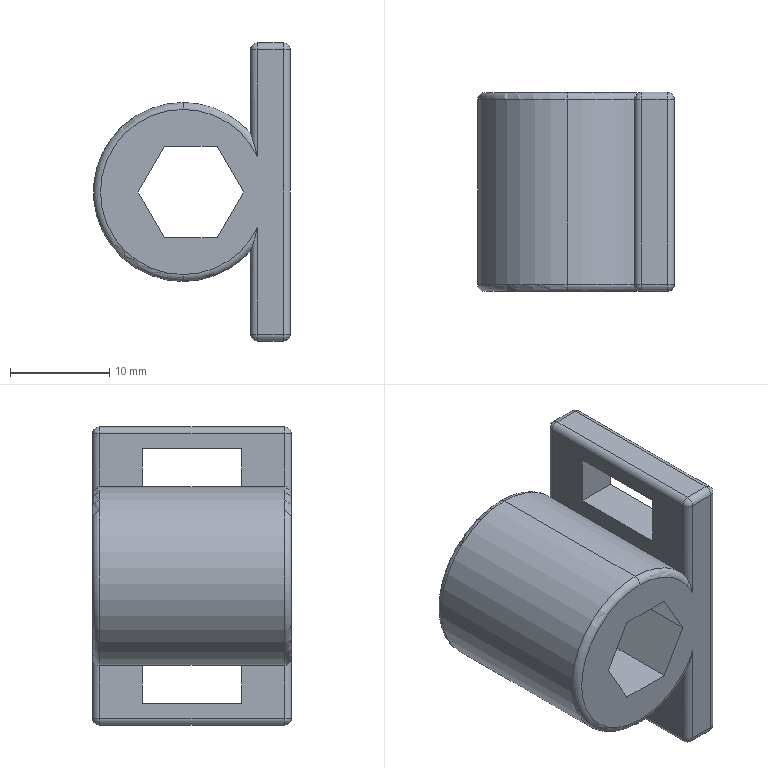Part | SolidWorks | features ICE 3, Fillet 2, Extrusion 1, MirrorPattern 1 | 1 solid | 52 faces | box 19.787 x 20 x 30 mm | volume 5242 mm3 | plane 21 | cylinder 17 | sphere 8 | torus 6 | commonest cylinder face diameters 1.4 x14 18 x3
STEP:
#1=CARTESIAN_POINT('',(-0.787,9.3,-9.));
#2=VERTEX_POINT('',#1);
#3=CARTESIAN_POINT('',(6.,9.3,-5.911));
#4=VERTEX_POINT('',#3);
#5=CARTESIAN_POINT('',(-0.787,9.3,0.));
#6=DIRECTION('',(0.,-1.,0.));
#7=DIRECTION('',(0.,0.,1.));
#8=AXIS2_PLACEMENT_3D('',#5,#6,#7);
#9=CIRCLE('',#8,9.);
#10=EDGE_CURVE('',#2,#4,#9,.T.);
#11=ORIENTED_EDGE('',*,*,#10,.F.);
#12=CARTESIAN_POINT('',(-0.787,10.,-8.3));
#13=VERTEX_POINT('',#12);
#14=CARTESIAN_POINT('',(-0.787,9.3,-8.3));
#15=DIRECTION('',(1.,0.,0.));
#16=DIRECTION('',(0.,0.,-1.));
#17=AXIS2_PLACEMENT_3D('',#14,#15,#16);
#18=CIRCLE('',#17,0.7);
#19=EDGE_CURVE('',#2,#13,#18,.T.);
#20=ORIENTED_EDGE('',*,*,#19,.T.);
#21=CARTESIAN_POINT('',(6.7,10.,-3.583));
#22=VERTEX_POINT('',#21);
#23=CARTESIAN_POINT('',(-0.787,10.,0.));
#24=DIRECTION('',(0.,1.,0.));
#25=DIRECTION('',(0.,0.,1.));
#26=AXIS2_PLACEMENT_3D('',#23,#24,#25);
#27=CIRCLE('',#26,8.3);
#28=EDGE_CURVE('',#22,#13,#27,.T.);
#29=ORIENTED_EDGE('',*,*,#28,.F.);
#30=CARTESIAN_POINT('',(6.,9.3,-5.911));
#31=CARTESIAN_POINT('',(6.,9.357,-5.911));
#32=CARTESIAN_POINT('',(6.007,9.412,-5.891));
#33=CARTESIAN_POINT('',(6.029,9.505,-5.833));
#34=CARTESIAN_POINT('',(6.043,9.545,-5.794));
#35=CARTESIAN_POINT('',(6.089,9.649,-5.67));
#36=CARTESIAN_POINT('',(6.123,9.699,-5.575));
#37=CARTESIAN_POINT('',(6.224,9.824,-5.283));
#38=CARTESIAN_POINT('',(6.293,9.874,-5.074));
#39=CARTESIAN_POINT('',(6.421,9.946,-4.656));
#40=CARTESIAN_POINT('',(6.482,9.968,-4.444));
#41=CARTESIAN_POINT('',(6.597,9.995,-4.016));
#42=CARTESIAN_POINT('',(6.65,10.,-3.802));
#43=CARTESIAN_POINT('',(6.7,10.,-3.583));
#44=B_SPLINE_CURVE_WITH_KNOTS('',3,(#30,#31,#32,#33,#34,#35,#36,#37,#38,#39,#40,#41,#42,#43),.UNSPECIFIED.,.F.,.F.,(4,2,2,2,2,2,4),(0.,0.0001684,0.0003368,0.0006737,0.001347,0.002021,0.002695),.UNSPECIFIED.);
#45=EDGE_CURVE('',#4,#22,#44,.T.);
#46=ORIENTED_EDGE('',*,*,#45,.F.);
#47=EDGE_LOOP('',(#11,#20,#29,#46));
#48=FACE_OUTER_BOUND('',#47,.T.);
#49=CARTESIAN_POINT('',(-0.787,9.3,0.));
#50=DIRECTION('',(0.,1.,0.));
#51=DIRECTION('',(0.,0.,1.));
#52=AXIS2_PLACEMENT_3D('',#49,#50,#51);
#53=TOROIDAL_SURFACE('',#52,8.3,0.7);
#54=ADVANCED_FACE('',(#48),#53,.T.);
#55=ORIENTED_EDGE('',*,*,#19,.F.);
#56=CARTESIAN_POINT('',(-0.787,9.3,9.));
#57=VERTEX_POINT('',#56);
#58=CARTESIAN_POINT('',(-0.787,9.3,0.));
#59=DIRECTION('',(0.,-1.,0.));
#60=DIRECTION('',(0.,0.,1.));
#61=AXIS2_PLACEMENT_3D('',#58,#59,#60);
#62=CIRCLE('',#61,9.);
#63=EDGE_CURVE('',#57,#2,#62,.T.);
#64=ORIENTED_EDGE('',*,*,#63,.F.);
#65=CARTESIAN_POINT('',(-0.787,10.,8.3));
#66=VERTEX_POINT('',#65);
#67=CARTESIAN_POINT('',(-0.787,9.3,8.3));
#68=DIRECTION('',(-1.,0.,0.));
#69=DIRECTION('',(0.,0.,1.));
#70=AXIS2_PLACEMENT_3D('',#67,#68,#69);
#71=CIRCLE('',#70,0.7);
#72=EDGE_CURVE('',#57,#66,#71,.T.);
#73=ORIENTED_EDGE('',*,*,#72,.T.);
#74=CARTESIAN_POINT('',(-0.787,10.,0.));
#75=DIRECTION('',(0.,1.,0.));
#76=DIRECTION('',(0.,0.,1.));
#77=AXIS2_PLACEMENT_3D('',#74,#75,#76);
#78=CIRCLE('',#77,8.3);
#79=EDGE_CURVE('',#13,#66,#78,.T.);
#80=ORIENTED_EDGE('',*,*,#79,.F.);
#81=EDGE_LOOP('',(#55,#64,#73,#80));
#82=FACE_OUTER_BOUND('',#81,.T.);
#83=CARTESIAN_POINT('',(-0.787,9.3,0.));
#84=DIRECTION('',(0.,1.,0.));
#85=DIRECTION('',(0.,0.,1.));
#86=AXIS2_PLACEMENT_3D('',#83,#84,#85);
#87=TOROIDAL_SURFACE('',#86,8.3,0.7);
#88=ADVANCED_FACE('',(#82),#87,.T.);
#89=CARTESIAN_POINT('',(-0.787,-10.,-8.3));
#90=VERTEX_POINT('',#89);
#91=CARTESIAN_POINT('',(6.7,-10.,-3.583));
#92=VERTEX_POINT('',#91);
#93=CARTESIAN_POINT('',(-0.787,-10.,0.));
#94=DIRECTION('',(0.,-1.,0.));
#95=DIRECTION('',(0.,0.,1.));
#96=AXIS2_PLACEMENT_3D('',#93,#94,#95);
#97=CIRCLE('',#96,8.3);
#98=EDGE_CURVE('',#90,#92,#97,.T.);
#99=ORIENTED_EDGE('',*,*,#98,.F.);
#100=CARTESIAN_POINT('',(-0.787,-9.3,-9.));
#101=VERTEX_POINT('',#100);
#102=CARTESIAN_POINT('',(-0.787,-9.3,-8.3));
#103=DIRECTION('',(1.,0.,0.));
#104=DIRECTION('',(0.,0.,-1.));
#105=AXIS2_PLACEMENT_3D('',#102,#103,#104);
#106=CIRCLE('',#105,0.7);
#107=EDGE_CURVE('',#90,#101,#106,.T.);
#108=ORIENTED_EDGE('',*,*,#107,.T.);
#109=CARTESIAN_POINT('',(6.,-9.3,-5.911));
#110=VERTEX_POINT('',#109);
#111=CARTESIAN_POINT('',(-0.787,-9.3,0.));
#112=DIRECTION('',(0.,1.,0.));
#113=DIRECTION('',(0.,0.,1.));
#114=AXIS2_PLACEMENT_3D('',#111,#112,#113);
#115=CIRCLE('',#114,9.);
#116=EDGE_CURVE('',#110,#101,#115,.T.);
#117=ORIENTED_EDGE('',*,*,#116,.F.);
#118=CARTESIAN_POINT('',(6.7,-10.,-3.583));
#119=CARTESIAN_POINT('',(6.601,-10.,-4.017));
#120=CARTESIAN_POINT('',(6.486,-9.983,-4.447));
#121=CARTESIAN_POINT('',(6.293,-9.874,-5.074));
#122=CARTESIAN_POINT('',(6.224,-9.824,-5.283));
#123=CARTESIAN_POINT('',(6.123,-9.699,-5.575));
#124=CARTESIAN_POINT('',(6.089,-9.649,-5.67));
#125=CARTESIAN_POINT('',(6.043,-9.545,-5.794));
#126=CARTESIAN_POINT('',(6.029,-9.505,-5.833));
#127=CARTESIAN_POINT('',(6.007,-9.412,-5.891));
#128=CARTESIAN_POINT('',(6.,-9.357,-5.911));
#129=CARTESIAN_POINT('',(6.,-9.3,-5.911));
#130=B_SPLINE_CURVE_WITH_KNOTS('',3,(#118,#119,#120,#121,#122,#123,#124,#125,#126,#127,#128,#129),.UNSPECIFIED.,.F.,.F.,(4,2,2,2,2,4),(-0.000008054,0.001327,0.001995,0.002329,0.002496,0.002663),.UNSPECIFIED.);
#131=EDGE_CURVE('',#92,#110,#130,.T.);
#132=ORIENTED_EDGE('',*,*,#131,.F.);
#133=EDGE_LOOP('',(#99,#108,#117,#132));
#134=FACE_OUTER_BOUND('',#133,.T.);
#135=CARTESIAN_POINT('',(-0.787,-9.3,0.));
#136=DIRECTION('',(0.,1.,0.));
#137=DIRECTION('',(0.,0.,1.));
#138=AXIS2_PLACEMENT_3D('',#135,#136,#137);
#139=TOROIDAL_SURFACE('',#138,8.3,0.7);
#140=ADVANCED_FACE('',(#134),#139,.T.);
#141=ORIENTED_EDGE('',*,*,#107,.F.);
#142=CARTESIAN_POINT('',(-0.787,-10.,8.3));
#143=VERTEX_POINT('',#142);
#144=CARTESIAN_POINT('',(-0.787,-10.,0.));
#145=DIRECTION('',(0.,-1.,0.));
#146=DIRECTION('',(0.,0.,1.));
#147=AXIS2_PLACEMENT_3D('',#144,#145,#146);
#148=CIRCLE('',#147,8.3);
#149=EDGE_CURVE('',#143,#90,#148,.T.);
#150=ORIENTED_EDGE('',*,*,#149,.F.);
#151=CARTESIAN_POINT('',(-0.787,-9.3,9.));
#152=VERTEX_POINT('',#151);
#153=CARTESIAN_POINT('',(-0.787,-9.3,8.3));
#154=DIRECTION('',(-1.,0.,0.));
#155=DIRECTION('',(0.,0.,1.));
#156=AXIS2_PLACEMENT_3D('',#153,#154,#155);
#157=CIRCLE('',#156,0.7);
#158=EDGE_CURVE('',#143,#152,#157,.T.);
#159=ORIENTED_EDGE('',*,*,#158,.T.);
#160=CARTESIAN_POINT('',(-0.787,-9.3,0.));
#161=DIRECTION('',(0.,1.,0.));
#162=DIRECTION('',(0.,0.,1.));
#163=AXIS2_PLACEMENT_3D('',#160,#161,#162);
#164=CIRCLE('',#163,9.);
#165=EDGE_CURVE('',#101,#152,#164,.T.);
#166=ORIENTED_EDGE('',*,*,#165,.F.);
#167=EDGE_LOOP('',(#141,#150,#159,#166));
#168=FACE_OUTER_BOUND('',#167,.T.);
#169=CARTESIAN_POINT('',(-0.787,-9.3,0.));
#170=DIRECTION('',(0.,1.,0.));
#171=DIRECTION('',(0.,0.,1.));
#172=AXIS2_PLACEMENT_3D('',#169,#170,#171);
#173=TOROIDAL_SURFACE('',#172,8.3,0.7);
#174=ADVANCED_FACE('',(#168),#173,.T.);
#175=ORIENTED_EDGE('',*,*,#116,.T.);
#176=CARTESIAN_POINT('',(-0.787,-10.,-9.));
#177=DIRECTION('',(0.,1.,0.));
#178=VECTOR('',#177,1000.);
#179=LINE('',#176,#178);
#180=EDGE_CURVE('',#101,#2,#179,.T.);
#181=ORIENTED_EDGE('',*,*,#180,.T.);
#182=ORIENTED_EDGE('',*,*,#10,.T.);
#183=CARTESIAN_POINT('',(6.,-10.,-5.911));
#184=DIRECTION('',(0.,1.,0.));
#185=VECTOR('',#184,1000.);
#186=LINE('',#183,#185);
#187=EDGE_CURVE('',#110,#4,#186,.T.);
#188=ORIENTED_EDGE('',*,*,#187,.F.);
#189=EDGE_LOOP('',(#175,#181,#182,#188));
#190=FACE_OUTER_BOUND('',#189,.T.);
#191=CARTESIAN_POINT('',(-0.787,-10.,0.));
#192=DIRECTION('',(0.,1.,0.));
#193=DIRECTION('',(0.,0.,1.));
#194=AXIS2_PLACEMENT_3D('',#191,#192,#193);
#195=CYLINDRICAL_SURFACE('',#194,9.);
#196=ADVANCED_FACE('',(#190),#195,.T.);
#197=ORIENTED_EDGE('',*,*,#180,.F.);
#198=ORIENTED_EDGE('',*,*,#165,.T.);
#199=CARTESIAN_POINT('',(-0.787,-10.,9.));
#200=DIRECTION('',(0.,1.,0.));
#201=VECTOR('',#200,1000.);
#202=LINE('',#199,#201);
#203=EDGE_CURVE('',#152,#57,#202,.T.);
#204=ORIENTED_EDGE('',*,*,#203,.T.);
#205=ORIENTED_EDGE('',*,*,#63,.T.);
#206=EDGE_LOOP('',(#197,#198,#204,#205));
#207=FACE_OUTER_BOUND('',#206,.T.);
#208=CARTESIAN_POINT('',(-0.787,-10.,0.));
#209=DIRECTION('',(0.,1.,0.));
#210=DIRECTION('',(0.,0.,1.));
#211=AXIS2_PLACEMENT_3D('',#208,#209,#210);
#212=CYLINDRICAL_SURFACE('',#211,9.);
#213=ADVANCED_FACE('',(#207),#212,.T.);
#214=CARTESIAN_POINT('',(10.,-9.3,-14.3));
#215=VERTEX_POINT('',#214);
#216=CARTESIAN_POINT('',(10.,9.3,-14.3));
#217=VERTEX_POINT('',#216);
#218=CARTESIAN_POINT('',(10.,10.,-14.3));
#219=DIRECTION('',(0.,1.,0.));
#220=VECTOR('',#219,1000.);
#221=LINE('',#218,#220);
#222=EDGE_CURVE('',#215,#217,#221,.T.);
#223=ORIENTED_EDGE('',*,*,#222,.T.);
#224=CARTESIAN_POINT('',(10.,9.3,14.3));
#225=VERTEX_POINT('',#224);
#226=CARTESIAN_POINT('',(10.,9.3,15.));
#227=DIRECTION('',(0.,0.,1.));
#228=VECTOR('',#227,1000.);
#229=LINE('',#226,#228);
#230=EDGE_CURVE('',#217,#225,#229,.T.);
#231=ORIENTED_EDGE('',*,*,#230,.T.);
#232=CARTESIAN_POINT('',(10.,-9.3,14.3));
#233=VERTEX_POINT('',#232);
#234=CARTESIAN_POINT('',(10.,10.,14.3));
#235=DIRECTION('',(0.,-1.,0.));
#236=VECTOR('',#235,1000.);
#237=LINE('',#234,#236);
#238=EDGE_CURVE('',#225,#233,#237,.T.);
#239=ORIENTED_EDGE('',*,*,#238,.T.);
#240=CARTESIAN_POINT('',(10.,-9.3,-15.));
#241=DIRECTION('',(0.,0.,-1.));
#242=VECTOR('',#241,1000.);
#243=LINE('',#240,#242);
#244=EDGE_CURVE('',#233,#215,#243,.T.);
#245=ORIENTED_EDGE('',*,*,#244,.T.);
#246=EDGE_LOOP('',(#223,#231,#239,#245));
#247=FACE_OUTER_BOUND('',#246,.T.);
#248=CARTESIAN_POINT('',(10.,5.,12.8));
#249=VERTEX_POINT('',#248);
#250=CARTESIAN_POINT('',(10.,5.,7.8));
#251=VERTEX_POINT('',#250);
#252=CARTESIAN_POINT('',(10.,5.,-15.));
#253=DIRECTION('',(0.,0.,-1.));
#254=VECTOR('',#253,1000.);
#255=LINE('',#252,#254);
#256=EDGE_CURVE('',#249,#251,#255,.T.);
#257=ORIENTED_EDGE('',*,*,#256,.T.);
#258=CARTESIAN_POINT('',(10.,-5.,7.8));
#259=VERTEX_POINT('',#258);
#260=CARTESIAN_POINT('',(10.,10.,7.8));
#261=DIRECTION('',(0.,-1.,0.));
#262=VECTOR('',#261,1000.);
#263=LINE('',#260,#262);
#264=EDGE_CURVE('',#251,#259,#263,.T.);
#265=ORIENTED_EDGE('',*,*,#264,.T.);
#266=CARTESIAN_POINT('',(10.,-5.,12.8));
#267=VERTEX_POINT('',#266);
#268=CARTESIAN_POINT('',(10.,-5.,-15.));
#269=DIRECTION('',(0.,0.,1.));
#270=VECTOR('',#269,1000.);
#271=LINE('',#268,#270);
#272=EDGE_CURVE('',#259,#267,#271,.T.);
#273=ORIENTED_EDGE('',*,*,#272,.T.);
#274=CARTESIAN_POINT('',(10.,10.,12.8));
#275=DIRECTION('',(0.,1.,0.));
#276=VECTOR('',#275,1000.);
#277=LINE('',#274,#276);
#278=EDGE_CURVE('',#267,#249,#277,.T.);
#279=ORIENTED_EDGE('',*,*,#278,.T.);
#280=EDGE_LOOP('',(#257,#265,#273,#279));
#281=FACE_BOUND('',#280,.T.);
#282=CARTESIAN_POINT('',(10.,5.,-7.8));
#283=VERTEX_POINT('',#282);
#284=CARTESIAN_POINT('',(10.,-5.,-7.8));
#285=VERTEX_POINT('',#284);
#286=CARTESIAN_POINT('',(10.,10.,-7.8));
#287=DIRECTION('',(0.,-1.,0.));
#288=VECTOR('',#287,1000.);
#289=LINE('',#286,#288);
#290=EDGE_CURVE('',#283,#285,#289,.T.);
#291=ORIENTED_EDGE('',*,*,#290,.F.);
#292=CARTESIAN_POINT('',(10.,5.,-12.8));
#293=VERTEX_POINT('',#292);
#294=CARTESIAN_POINT('',(10.,5.,-15.));
#295=DIRECTION('',(0.,0.,1.));
#296=VECTOR('',#295,1000.);
#297=LINE('',#294,#296);
#298=EDGE_CURVE('',#293,#283,#297,.T.);
#299=ORIENTED_EDGE('',*,*,#298,.F.);
#300=CARTESIAN_POINT('',(10.,-5.,-12.8));
#301=VERTEX_POINT('',#300);
#302=CARTESIAN_POINT('',(10.,10.,-12.8));
#303=DIRECTION('',(0.,1.,0.));
#304=VECTOR('',#303,1000.);
#305=LINE('',#302,#304);
#306=EDGE_CURVE('',#301,#293,#305,.T.);
#307=ORIENTED_EDGE('',*,*,#306,.F.);
#308=CARTESIAN_POINT('',(10.,-5.,-15.));
#309=DIRECTION('',(0.,0.,-1.));
#310=VECTOR('',#309,1000.);
#311=LINE('',#308,#310);
#312=EDGE_CURVE('',#285,#301,#311,.T.);
#313=ORIENTED_EDGE('',*,*,#312,.F.);
#314=EDGE_LOOP('',(#291,#299,#307,#313));
#315=FACE_BOUND('',#314,.T.);
#316=CARTESIAN_POINT('',(10.,10.,-15.));
#317=DIRECTION('',(-1.,0.,0.));
#318=DIRECTION('',(0.,0.,1.));
#319=AXIS2_PLACEMENT_3D('',#316,#317,#318);
#320=PLANE('',#319);
#321=ADVANCED_FACE('',(#247,#281,#315),#320,.F.);
#322=CARTESIAN_POINT('',(6.,9.3,-14.3));
#323=VERTEX_POINT('',#322);
#324=CARTESIAN_POINT('',(6.,-9.3,-14.3));
#325=VERTEX_POINT('',#324);
#326=CARTESIAN_POINT('',(6.,-10.,-14.3));
#327=DIRECTION('',(0.,-1.,0.));
#328=VECTOR('',#327,1000.);
#329=LINE('',#326,#328);
#330=EDGE_CURVE('',#323,#325,#329,.T.);
#331=ORIENTED_EDGE('',*,*,#330,.T.);
#332=CARTESIAN_POINT('',(6.,-9.3,-5.911));
#333=DIRECTION('',(0.,0.,1.));
#334=VECTOR('',#333,1000.);
#335=LINE('',#332,#334);
#336=EDGE_CURVE('',#325,#110,#335,.T.);
#337=ORIENTED_EDGE('',*,*,#336,.T.);
#338=ORIENTED_EDGE('',*,*,#187,.T.);
#339=CARTESIAN_POINT('',(6.,9.3,-5.911));
#340=DIRECTION('',(0.,0.,-1.));
#341=VECTOR('',#340,1000.);
#342=LINE('',#339,#341);
#343=EDGE_CURVE('',#4,#323,#342,.T.);
#344=ORIENTED_EDGE('',*,*,#343,.T.);
#345=EDGE_LOOP('',(#331,#337,#338,#344));
#346=FACE_OUTER_BOUND('',#345,.T.);
#347=CARTESIAN_POINT('',(6.,5.,-12.8));
#348=VERTEX_POINT('',#347);
#349=CARTESIAN_POINT('',(6.,5.,-7.8));
#350=VERTEX_POINT('',#349);
#351=CARTESIAN_POINT('',(6.,5.,-7.8));
#352=DIRECTION('',(0.,0.,1.));
#353=VECTOR('',#352,1000.);
#354=LINE('',#351,#353);
#355=EDGE_CURVE('',#348,#350,#354,.T.);
#356=ORIENTED_EDGE('',*,*,#355,.T.);
#357=CARTESIAN_POINT('',(6.,-5.,-7.8));
#358=VERTEX_POINT('',#357);
#359=CARTESIAN_POINT('',(6.,5.,-7.8));
#360=DIRECTION('',(0.,-1.,0.));
#361=VECTOR('',#360,1000.);
#362=LINE('',#359,#361);
#363=EDGE_CURVE('',#350,#358,#362,.T.);
#364=ORIENTED_EDGE('',*,*,#363,.T.);
#365=CARTESIAN_POINT('',(6.,-5.,-12.8));
#366=VERTEX_POINT('',#365);
#367=CARTESIAN_POINT('',(6.,-5.,-7.8));
#368=DIRECTION('',(0.,0.,-1.));
#369=VECTOR('',#368,1000.);
#370=LINE('',#367,#369);
#371=EDGE_CURVE('',#358,#366,#370,.T.);
#372=ORIENTED_EDGE('',*,*,#371,.T.);
#373=CARTESIAN_POINT('',(6.,5.,-12.8));
#374=DIRECTION('',(0.,1.,0.));
#375=VECTOR('',#374,1000.);
#376=LINE('',#373,#375);
#377=EDGE_CURVE('',#366,#348,#376,.T.);
#378=ORIENTED_EDGE('',*,*,#377,.T.);
#379=EDGE_LOOP('',(#356,#364,#372,#378));
#380=FACE_BOUND('',#379,.T.);
#381=CARTESIAN_POINT('',(6.,-10.,-5.911));
#382=DIRECTION('',(-1.,0.,0.));
#383=DIRECTION('',(0.,0.,1.));
#384=AXIS2_PLACEMENT_3D('',#381,#382,#383);
#385=PLANE('',#384);
#386=ADVANCED_FACE('',(#346,#380),#385,.T.);
#387=CARTESIAN_POINT('',(9.3,9.3,-15.));
#388=VERTEX_POINT('',#387);
#389=CARTESIAN_POINT('',(9.3,-9.3,-15.));
#390=VERTEX_POINT('',#389);
#391=CARTESIAN_POINT('',(9.3,10.,-15.));
#392=DIRECTION('',(0.,-1.,0.));
#393=VECTOR('',#392,1000.);
#394=LINE('',#391,#393);
#395=EDGE_CURVE('',#388,#390,#394,.T.);
#396=ORIENTED_EDGE('',*,*,#395,.T.);
#397=CARTESIAN_POINT('',(6.7,-9.3,-15.));
#398=VERTEX_POINT('',#397);
#399=CARTESIAN_POINT('',(-10.,-9.3,-15.));
#400=DIRECTION('',(-1.,0.,0.));
#401=VECTOR('',#400,1000.);
#402=LINE('',#399,#401);
#403=EDGE_CURVE('',#390,#398,#402,.T.);
#404=ORIENTED_EDGE('',*,*,#403,.T.);
#405=CARTESIAN_POINT('',(6.7,9.3,-15.));
#406=VERTEX_POINT('',#405);
#407=CARTESIAN_POINT('',(6.7,10.,-15.));
#408=DIRECTION('',(0.,1.,0.));
#409=VECTOR('',#408,1000.);
#410=LINE('',#407,#409);
#411=EDGE_CURVE('',#398,#406,#410,.T.);
#412=ORIENTED_EDGE('',*,*,#411,.T.);
#413=CARTESIAN_POINT('',(10.,9.3,-15.));
#414=DIRECTION('',(1.,0.,0.));
#415=VECTOR('',#414,1000.);
#416=LINE('',#413,#415);
#417=EDGE_CURVE('',#406,#388,#416,.T.);
#418=ORIENTED_EDGE('',*,*,#417,.T.);
#419=EDGE_LOOP('',(#396,#404,#412,#418));
#420=FACE_OUTER_BOUND('',#419,.T.);
#421=CARTESIAN_POINT('',(-10.,10.,-15.));
#422=DIRECTION('',(0.,0.,1.));
#423=DIRECTION('',(1.,0.,0.));
#424=AXIS2_PLACEMENT_3D('',#421,#422,#423);
#425=PLANE('',#424);
#426=ADVANCED_FACE('',(#420),#425,.F.);
#427=CARTESIAN_POINT('',(6.7,-9.3,15.));
#428=VERTEX_POINT('',#427);
#429=CARTESIAN_POINT('',(9.3,-9.3,15.));
#430=VERTEX_POINT('',#429);
#431=CARTESIAN_POINT('',(-10.,-9.3,15.));
#432=DIRECTION('',(1.,0.,0.));
#433=VECTOR('',#432,1000.);
#434=LINE('',#431,#433);
#435=EDGE_CURVE('',#428,#430,#434,.T.);
#436=ORIENTED_EDGE('',*,*,#435,.T.);
#437=CARTESIAN_POINT('',(9.3,9.3,15.));
#438=VERTEX_POINT('',#437);
#439=CARTESIAN_POINT('',(9.3,10.,15.));
#440=DIRECTION('',(0.,1.,0.));
#441=VECTOR('',#440,1000.);
#442=LINE('',#439,#441);
#443=EDGE_CURVE('',#430,#438,#442,.T.);
#444=ORIENTED_EDGE('',*,*,#443,.T.);
#445=CARTESIAN_POINT('',(6.7,9.3,15.));
#446=VERTEX_POINT('',#445);
#447=CARTESIAN_POINT('',(6.,9.3,15.));
#448=DIRECTION('',(-1.,0.,0.));
#449=VECTOR('',#448,1000.);
#450=LINE('',#447,#449);
#451=EDGE_CURVE('',#438,#446,#450,.T.);
#452=ORIENTED_EDGE('',*,*,#451,.T.);
#453=CARTESIAN_POINT('',(6.7,-10.,15.));
#454=DIRECTION('',(0.,-1.,0.));
#455=VECTOR('',#454,1000.);
#456=LINE('',#453,#455);
#457=EDGE_CURVE('',#446,#428,#456,.T.);
#458=ORIENTED_EDGE('',*,*,#457,.T.);
#459=EDGE_LOOP('',(#436,#444,#452,#458));
#460=FACE_OUTER_BOUND('',#459,.T.);
#461=CARTESIAN_POINT('',(-10.,10.,15.));
#462=DIRECTION('',(0.,0.,-1.));
#463=DIRECTION('',(-1.,0.,0.));
#464=AXIS2_PLACEMENT_3D('',#461,#462,#463);
#465=PLANE('',#464);
#466=ADVANCED_FACE('',(#460),#465,.F.);
#467=CARTESIAN_POINT('',(2.65,10.,4.59));
#468=VERTEX_POINT('',#467);
#469=CARTESIAN_POINT('',(5.3,10.,0.));
#470=VERTEX_POINT('',#469);
#471=CARTESIAN_POINT('',(2.65,10.,4.59));
#472=DIRECTION('',(0.5,0.,-0.866));
#473=VECTOR('',#472,1000.);
#474=LINE('',#471,#473);
#475=EDGE_CURVE('',#468,#470,#474,.T.);
#476=ORIENTED_EDGE('',*,*,#475,.F.);
#477=CARTESIAN_POINT('',(-2.65,10.,4.59));
#478=VERTEX_POINT('',#477);
#479=CARTESIAN_POINT('',(-2.65,10.,4.59));
#480=DIRECTION('',(1.,0.,0.));
#481=VECTOR('',#480,1000.);
#482=LINE('',#479,#481);
#483=EDGE_CURVE('',#478,#468,#482,.T.);
#484=ORIENTED_EDGE('',*,*,#483,.F.);
#485=CARTESIAN_POINT('',(-5.3,10.,0.));
#486=VERTEX_POINT('',#485);
#487=CARTESIAN_POINT('',(-5.3,10.,0.));
#488=DIRECTION('',(0.5,0.,0.866));
#489=VECTOR('',#488,1000.);
#490=LINE('',#487,#489);
#491=EDGE_CURVE('',#486,#478,#490,.T.);
#492=ORIENTED_EDGE('',*,*,#491,.F.);
#493=CARTESIAN_POINT('',(-2.65,10.,-4.59));
#494=VERTEX_POINT('',#493);
#495=CARTESIAN_POINT('',(-2.65,10.,-4.59));
#496=DIRECTION('',(-0.5,0.,0.866));
#497=VECTOR('',#496,1000.);
#498=LINE('',#495,#497);
#499=EDGE_CURVE('',#494,#486,#498,.T.);
#500=ORIENTED_EDGE('',*,*,#499,.F.);
#501=CARTESIAN_POINT('',(2.65,10.,-4.59));
#502=VERTEX_POINT('',#501);
#503=CARTESIAN_POINT('',(2.65,10.,-4.59));
#504=DIRECTION('',(-1.,0.,0.));
#505=VECTOR('',#504,1000.);
#506=LINE('',#503,#505);
#507=EDGE_CURVE('',#502,#494,#506,.T.);
#508=ORIENTED_EDGE('',*,*,#507,.F.);
#509=CARTESIAN_POINT('',(5.3,10.,0.));
#510=DIRECTION('',(-0.5,0.,-0.866));
#511=VECTOR('',#510,1000.);
#512=LINE('',#509,#511);
#513=EDGE_CURVE('',#470,#502,#512,.T.);
#514=ORIENTED_EDGE('',*,*,#513,.F.);
#515=EDGE_LOOP('',(#476,#484,#492,#500,#508,#514));
#516=FACE_BOUND('',#515,.T.);
#517=ORIENTED_EDGE('',*,*,#28,.T.);
#518=ORIENTED_EDGE('',*,*,#79,.T.);
#519=CARTESIAN_POINT('',(6.7,10.,3.583));
#520=VERTEX_POINT('',#519);
#521=CARTESIAN_POINT('',(-0.787,10.,0.));
#522=DIRECTION('',(0.,1.,0.));
#523=DIRECTION('',(0.,0.,1.));
#524=AXIS2_PLACEMENT_3D('',#521,#522,#523);
#525=CIRCLE('',#524,8.3);
#526=EDGE_CURVE('',#66,#520,#525,.T.);
#527=ORIENTED_EDGE('',*,*,#526,.T.);
#528=CARTESIAN_POINT('',(6.7,10.,14.3));
#529=VERTEX_POINT('',#528);
#530=CARTESIAN_POINT('',(6.7,10.,0.));
#531=DIRECTION('',(0.,0.,1.));
#532=VECTOR('',#531,1000.);
#533=LINE('',#530,#532);
#534=EDGE_CURVE('',#520,#529,#533,.T.);
#535=ORIENTED_EDGE('',*,*,#534,.T.);
#536=CARTESIAN_POINT('',(9.3,10.,14.3));
#537=VERTEX_POINT('',#536);
#538=CARTESIAN_POINT('',(10.,10.,14.3));
#539=DIRECTION('',(1.,0.,0.));
#540=VECTOR('',#539,1000.);
#541=LINE('',#538,#540);
#542=EDGE_CURVE('',#529,#537,#541,.T.);
#543=ORIENTED_EDGE('',*,*,#542,.T.);
#544=CARTESIAN_POINT('',(9.3,10.,-14.3));
#545=VERTEX_POINT('',#544);
#546=CARTESIAN_POINT('',(9.3,10.,-15.));
#547=DIRECTION('',(0.,0.,-1.));
#548=VECTOR('',#547,1000.);
#549=LINE('',#546,#548);
#550=EDGE_CURVE('',#537,#545,#549,.T.);
#551=ORIENTED_EDGE('',*,*,#550,.T.);
#552=CARTESIAN_POINT('',(6.7,10.,-14.3));
#553=VERTEX_POINT('',#552);
#554=CARTESIAN_POINT('',(6.,10.,-14.3));
#555=DIRECTION('',(-1.,0.,0.));
#556=VECTOR('',#555,1000.);
#557=LINE('',#554,#556);
#558=EDGE_CURVE('',#545,#553,#557,.T.);
#559=ORIENTED_EDGE('',*,*,#558,.T.);
#560=CARTESIAN_POINT('',(6.7,10.,0.));
#561=DIRECTION('',(0.,0.,1.));
#562=VECTOR('',#561,1000.);
#563=LINE('',#560,#562);
#564=EDGE_CURVE('',#553,#22,#563,.T.);
#565=ORIENTED_EDGE('',*,*,#564,.T.);
#566=EDGE_LOOP('',(#517,#518,#527,#535,#543,#551,#559,#565));
#567=FACE_OUTER_BOUND('',#566,.T.);
#568=CARTESIAN_POINT('',(0.,10.,0.));
#569=DIRECTION('',(0.,1.,0.));
#570=DIRECTION('',(0.,0.,1.));
#571=AXIS2_PLACEMENT_3D('',#568,#569,#570);
#572=PLANE('',#571);
#573=ADVANCED_FACE('',(#516,#567),#572,.T.);
#574=CARTESIAN_POINT('',(2.65,-10.,4.59));
#575=VERTEX_POINT('',#574);
#576=CARTESIAN_POINT('',(-2.65,-10.,4.59));
#577=VERTEX_POINT('',#576);
#578=CARTESIAN_POINT('',(-2.65,-10.,4.59));
#579=DIRECTION('',(-1.,0.,0.));
#580=VECTOR('',#579,1000.);
#581=LINE('',#578,#580);
#582=EDGE_CURVE('',#575,#577,#581,.T.);
#583=ORIENTED_EDGE('',*,*,#582,.F.);
#584=CARTESIAN_POINT('',(5.3,-10.,0.));
#585=VERTEX_POINT('',#584);
#586=CARTESIAN_POINT('',(2.65,-10.,4.59));
#587=DIRECTION('',(-0.5,0.,0.866));
#588=VECTOR('',#587,1000.);
#589=LINE('',#586,#588);
#590=EDGE_CURVE('',#585,#575,#589,.T.);
#591=ORIENTED_EDGE('',*,*,#590,.F.);
#592=CARTESIAN_POINT('',(2.65,-10.,-4.59));
#593=VERTEX_POINT('',#592);
#594=CARTESIAN_POINT('',(5.3,-10.,0.));
#595=DIRECTION('',(0.5,0.,0.866));
#596=VECTOR('',#595,1000.);
#597=LINE('',#594,#596);
#598=EDGE_CURVE('',#593,#585,#597,.T.);
#599=ORIENTED_EDGE('',*,*,#598,.F.);
#600=CARTESIAN_POINT('',(-2.65,-10.,-4.59));
#601=VERTEX_POINT('',#600);
#602=CARTESIAN_POINT('',(2.65,-10.,-4.59));
#603=DIRECTION('',(1.,0.,0.));
#604=VECTOR('',#603,1000.);
#605=LINE('',#602,#604);
#606=EDGE_CURVE('',#601,#593,#605,.T.);
#607=ORIENTED_EDGE('',*,*,#606,.F.);
#608=CARTESIAN_POINT('',(-5.3,-10.,0.));
#609=VERTEX_POINT('',#608);
#610=CARTESIAN_POINT('',(-2.65,-10.,-4.59));
#611=DIRECTION('',(0.5,0.,-0.866));
#612=VECTOR('',#611,1000.);
#613=LINE('',#610,#612);
#614=EDGE_CURVE('',#609,#601,#613,.T.);
#615=ORIENTED_EDGE('',*,*,#614,.F.);
#616=CARTESIAN_POINT('',(-5.3,-10.,0.));
#617=DIRECTION('',(-0.5,0.,-0.866));
#618=VECTOR('',#617,1000.);
#619=LINE('',#616,#618);
#620=EDGE_CURVE('',#577,#609,#619,.T.);
#621=ORIENTED_EDGE('',*,*,#620,.F.);
#622=EDGE_LOOP('',(#583,#591,#599,#607,#615,#621));
#623=FACE_BOUND('',#622,.T.);
#624=CARTESIAN_POINT('',(6.7,-10.,14.3));
#625=VERTEX_POINT('',#624);
#626=CARTESIAN_POINT('',(6.7,-10.,3.583));
#627=VERTEX_POINT('',#626);
#628=CARTESIAN_POINT('',(6.7,-10.,5.911));
#629=DIRECTION('',(0.,0.,-1.));
#630=VECTOR('',#629,1000.);
#631=LINE('',#628,#630);
#632=EDGE_CURVE('',#625,#627,#631,.T.);
#633=ORIENTED_EDGE('',*,*,#632,.T.);
#634=CARTESIAN_POINT('',(-0.787,-10.,0.));
#635=DIRECTION('',(0.,-1.,0.));
#636=DIRECTION('',(0.,0.,1.));
#637=AXIS2_PLACEMENT_3D('',#634,#635,#636);
#638=CIRCLE('',#637,8.3);
#639=EDGE_CURVE('',#627,#143,#638,.T.);
#640=ORIENTED_EDGE('',*,*,#639,.T.);
#641=ORIENTED_EDGE('',*,*,#149,.T.);
#642=ORIENTED_EDGE('',*,*,#98,.T.);
#643=CARTESIAN_POINT('',(6.7,-10.,-14.3));
#644=VERTEX_POINT('',#643);
#645=CARTESIAN_POINT('',(6.7,-10.,-15.));
#646=DIRECTION('',(0.,0.,-1.));
#647=VECTOR('',#646,1000.);
#648=LINE('',#645,#647);
#649=EDGE_CURVE('',#92,#644,#648,.T.);
#650=ORIENTED_EDGE('',*,*,#649,.T.);
#651=CARTESIAN_POINT('',(9.3,-10.,-14.3));
#652=VERTEX_POINT('',#651);
#653=CARTESIAN_POINT('',(0.,-10.,-14.3));
#654=DIRECTION('',(1.,0.,0.));
#655=VECTOR('',#654,1000.);
#656=LINE('',#653,#655);
#657=EDGE_CURVE('',#644,#652,#656,.T.);
#658=ORIENTED_EDGE('',*,*,#657,.T.);
#659=CARTESIAN_POINT('',(9.3,-10.,14.3));
#660=VERTEX_POINT('',#659);
#661=CARTESIAN_POINT('',(9.3,-10.,0.));
#662=DIRECTION('',(0.,0.,1.));
#663=VECTOR('',#662,1000.);
#664=LINE('',#661,#663);
#665=EDGE_CURVE('',#652,#660,#664,.T.);
#666=ORIENTED_EDGE('',*,*,#665,.T.);
#667=CARTESIAN_POINT('',(0.,-10.,14.3));
#668=DIRECTION('',(-1.,0.,0.));
#669=VECTOR('',#668,1000.);
#670=LINE('',#667,#669);
#671=EDGE_CURVE('',#660,#625,#670,.T.);
#672=ORIENTED_EDGE('',*,*,#671,.T.);
#673=EDGE_LOOP('',(#633,#640,#641,#642,#650,#658,#666,#672));
#674=FACE_OUTER_BOUND('',#673,.T.);
#675=CARTESIAN_POINT('',(0.,-10.,0.));
#676=DIRECTION('',(0.,1.,0.));
#677=DIRECTION('',(0.,0.,1.));
#678=AXIS2_PLACEMENT_3D('',#675,#676,#677);
#679=PLANE('',#678);
#680=ADVANCED_FACE('',(#623,#674),#679,.F.);
#681=ORIENTED_EDGE('',*,*,#590,.T.);
#682=CARTESIAN_POINT('',(2.65,-10.001,4.59));
#683=DIRECTION('',(0.,1.,0.));
#684=VECTOR('',#683,1000.);
#685=LINE('',#682,#684);
#686=EDGE_CURVE('',#575,#468,#685,.T.);
#687=ORIENTED_EDGE('',*,*,#686,.T.);
#688=ORIENTED_EDGE('',*,*,#475,.T.);
#689=CARTESIAN_POINT('',(5.3,-10.001,0.));
#690=DIRECTION('',(0.,1.,0.));
#691=VECTOR('',#690,1000.);
#692=LINE('',#689,#691);
#693=EDGE_CURVE('',#585,#470,#692,.T.);
#694=ORIENTED_EDGE('',*,*,#693,.F.);
#695=EDGE_LOOP('',(#681,#687,#688,#694));
#696=FACE_OUTER_BOUND('',#695,.T.);
#697=CARTESIAN_POINT('',(2.65,-10.001,4.59));
#698=DIRECTION('',(0.866,0.,0.5));
#699=DIRECTION('',(0.5,0.,-0.866));
#700=AXIS2_PLACEMENT_3D('',#697,#698,#699);
#701=PLANE('',#700);
#702=ADVANCED_FACE('',(#696),#701,.F.);
#703=ORIENTED_EDGE('',*,*,#582,.T.);
#704=CARTESIAN_POINT('',(-2.65,-10.001,4.59));
#705=DIRECTION('',(0.,1.,0.));
#706=VECTOR('',#705,1000.);
#707=LINE('',#704,#706);
#708=EDGE_CURVE('',#577,#478,#707,.T.);
#709=ORIENTED_EDGE('',*,*,#708,.T.);
#710=ORIENTED_EDGE('',*,*,#483,.T.);
#711=ORIENTED_EDGE('',*,*,#686,.F.);
#712=EDGE_LOOP('',(#703,#709,#710,#711));
#713=FACE_OUTER_BOUND('',#712,.T.);
#714=CARTESIAN_POINT('',(-2.65,-10.001,4.59));
#715=DIRECTION('',(0.,0.,1.));
#716=DIRECTION('',(1.,0.,0.));
#717=AXIS2_PLACEMENT_3D('',#714,#715,#716);
#718=PLANE('',#717);
#719=ADVANCED_FACE('',(#713),#718,.F.);
#720=ORIENTED_EDGE('',*,*,#620,.T.);
#721=CARTESIAN_POINT('',(-5.3,-10.001,0.));
#722=DIRECTION('',(0.,1.,0.));
#723=VECTOR('',#722,1000.);
#724=LINE('',#721,#723);
#725=EDGE_CURVE('',#609,#486,#724,.T.);
#726=ORIENTED_EDGE('',*,*,#725,.T.);
#727=ORIENTED_EDGE('',*,*,#491,.T.);
#728=ORIENTED_EDGE('',*,*,#708,.F.);
#729=EDGE_LOOP('',(#720,#726,#727,#728));
#730=FACE_OUTER_BOUND('',#729,.T.);
#731=CARTESIAN_POINT('',(-5.3,-10.001,0.));
#732=DIRECTION('',(-0.866,0.,0.5));
#733=DIRECTION('',(0.5,0.,0.866));
#734=AXIS2_PLACEMENT_3D('',#731,#732,#733);
#735=PLANE('',#734);
#736=ADVANCED_FACE('',(#730),#735,.F.);
#737=ORIENTED_EDGE('',*,*,#614,.T.);
#738=CARTESIAN_POINT('',(-2.65,-10.001,-4.59));
#739=DIRECTION('',(0.,1.,0.));
#740=VECTOR('',#739,1000.);
#741=LINE('',#738,#740);
#742=EDGE_CURVE('',#601,#494,#741,.T.);
#743=ORIENTED_EDGE('',*,*,#742,.T.);
#744=ORIENTED_EDGE('',*,*,#499,.T.);
#745=ORIENTED_EDGE('',*,*,#725,.F.);
#746=EDGE_LOOP('',(#737,#743,#744,#745));
#747=FACE_OUTER_BOUND('',#746,.T.);
#748=CARTESIAN_POINT('',(-2.65,-10.001,-4.59));
#749=DIRECTION('',(-0.866,0.,-0.5));
#750=DIRECTION('',(-0.5,0.,0.866));
#751=AXIS2_PLACEMENT_3D('',#748,#749,#750);
#752=PLANE('',#751);
#753=ADVANCED_FACE('',(#747),#752,.F.);
#754=ORIENTED_EDGE('',*,*,#606,.T.);
#755=CARTESIAN_POINT('',(2.65,-10.001,-4.59));
#756=DIRECTION('',(0.,1.,0.));
#757=VECTOR('',#756,1000.);
#758=LINE('',#755,#757);
#759=EDGE_CURVE('',#593,#502,#758,.T.);
#760=ORIENTED_EDGE('',*,*,#759,.T.);
#761=ORIENTED_EDGE('',*,*,#507,.T.);
#762=ORIENTED_EDGE('',*,*,#742,.F.);
#763=EDGE_LOOP('',(#754,#760,#761,#762));
#764=FACE_OUTER_BOUND('',#763,.T.);
#765=CARTESIAN_POINT('',(2.65,-10.001,-4.59));
#766=DIRECTION('',(0.,0.,-1.));
#767=DIRECTION('',(-1.,0.,0.));
#768=AXIS2_PLACEMENT_3D('',#765,#766,#767);
#769=PLANE('',#768);
#770=ADVANCED_FACE('',(#764),#769,.F.);
#771=ORIENTED_EDGE('',*,*,#598,.T.);
#772=ORIENTED_EDGE('',*,*,#693,.T.);
#773=ORIENTED_EDGE('',*,*,#513,.T.);
#774=ORIENTED_EDGE('',*,*,#759,.F.);
#775=EDGE_LOOP('',(#771,#772,#773,#774));
#776=FACE_OUTER_BOUND('',#775,.T.);
#777=CARTESIAN_POINT('',(5.3,-10.001,0.));
#778=DIRECTION('',(0.866,0.,-0.5));
#779=DIRECTION('',(-0.5,0.,-0.866));
#780=AXIS2_PLACEMENT_3D('',#777,#778,#779);
#781=PLANE('',#780);
#782=ADVANCED_FACE('',(#776),#781,.F.);
#783=CARTESIAN_POINT('',(6.,5.,7.8));
#784=VERTEX_POINT('',#783);
#785=CARTESIAN_POINT('',(6.,-5.,7.8));
#786=VERTEX_POINT('',#785);
#787=CARTESIAN_POINT('',(6.,5.,7.8));
#788=DIRECTION('',(0.,-1.,0.));
#789=VECTOR('',#788,1000.);
#790=LINE('',#787,#789);
#791=EDGE_CURVE('',#784,#786,#790,.T.);
#792=ORIENTED_EDGE('',*,*,#791,.F.);
#793=CARTESIAN_POINT('',(6.,5.,12.8));
#794=VERTEX_POINT('',#793);
#795=CARTESIAN_POINT('',(6.,5.,7.8));
#796=DIRECTION('',(0.,0.,-1.));
#797=VECTOR('',#796,1000.);
#798=LINE('',#795,#797);
#799=EDGE_CURVE('',#794,#784,#798,.T.);
#800=ORIENTED_EDGE('',*,*,#799,.F.);
#801=CARTESIAN_POINT('',(6.,-5.,12.8));
#802=VERTEX_POINT('',#801);
#803=CARTESIAN_POINT('',(6.,5.,12.8));
#804=DIRECTION('',(0.,1.,0.));
#805=VECTOR('',#804,1000.);
#806=LINE('',#803,#805);
#807=EDGE_CURVE('',#802,#794,#806,.T.);
#808=ORIENTED_EDGE('',*,*,#807,.F.);
#809=CARTESIAN_POINT('',(6.,-5.,7.8));
#810=DIRECTION('',(0.,0.,1.));
#811=VECTOR('',#810,1000.);
#812=LINE('',#809,#811);
#813=EDGE_CURVE('',#786,#802,#812,.T.);
#814=ORIENTED_EDGE('',*,*,#813,.F.);
#815=EDGE_LOOP('',(#792,#800,#808,#814));
#816=FACE_BOUND('',#815,.T.);
#817=CARTESIAN_POINT('',(6.,-9.3,14.3));
#818=VERTEX_POINT('',#817);
#819=CARTESIAN_POINT('',(6.,9.3,14.3));
#820=VERTEX_POINT('',#819);
#821=CARTESIAN_POINT('',(6.,10.,14.3));
#822=DIRECTION('',(0.,1.,0.));
#823=VECTOR('',#822,1000.);
#824=LINE('',#821,#823);
#825=EDGE_CURVE('',#818,#820,#824,.T.);
#826=ORIENTED_EDGE('',*,*,#825,.T.);
#827=CARTESIAN_POINT('',(6.,9.3,5.911));
#828=VERTEX_POINT('',#827);
#829=CARTESIAN_POINT('',(6.,9.3,15.));
#830=DIRECTION('',(0.,0.,-1.));
#831=VECTOR('',#830,1000.);
#832=LINE('',#829,#831);
#833=EDGE_CURVE('',#820,#828,#832,.T.);
#834=ORIENTED_EDGE('',*,*,#833,.T.);
#835=CARTESIAN_POINT('',(6.,-9.3,5.911));
#836=VERTEX_POINT('',#835);
#837=CARTESIAN_POINT('',(6.,-10.,5.911));
#838=DIRECTION('',(0.,1.,0.));
#839=VECTOR('',#838,1000.);
#840=LINE('',#837,#839);
#841=EDGE_CURVE('',#836,#828,#840,.T.);
#842=ORIENTED_EDGE('',*,*,#841,.F.);
#843=CARTESIAN_POINT('',(6.,-9.3,15.));
#844=DIRECTION('',(0.,0.,1.));
#845=VECTOR('',#844,1000.);
#846=LINE('',#843,#845);
#847=EDGE_CURVE('',#836,#818,#846,.T.);
#848=ORIENTED_EDGE('',*,*,#847,.T.);
#849=EDGE_LOOP('',(#826,#834,#842,#848));
#850=FACE_OUTER_BOUND('',#849,.T.);
#851=CARTESIAN_POINT('',(6.,-10.,15.));
#852=DIRECTION('',(-1.,0.,0.));
#853=DIRECTION('',(0.,0.,1.));
#854=AXIS2_PLACEMENT_3D('',#851,#852,#853);
#855=PLANE('',#854);
#856=ADVANCED_FACE('',(#816,#850),#855,.T.);
#857=ORIENTED_EDGE('',*,*,#203,.F.);
#858=CARTESIAN_POINT('',(-0.787,-9.3,0.));
#859=DIRECTION('',(0.,1.,0.));
#860=DIRECTION('',(0.,0.,1.));
#861=AXIS2_PLACEMENT_3D('',#858,#859,#860);
#862=CIRCLE('',#861,9.);
#863=EDGE_CURVE('',#152,#836,#862,.T.);
#864=ORIENTED_EDGE('',*,*,#863,.T.);
#865=ORIENTED_EDGE('',*,*,#841,.T.);
#866=CARTESIAN_POINT('',(-0.787,9.3,0.));
#867=DIRECTION('',(0.,-1.,0.));
#868=DIRECTION('',(0.,0.,1.));
#869=AXIS2_PLACEMENT_3D('',#866,#867,#868);
#870=CIRCLE('',#869,9.);
#871=EDGE_CURVE('',#828,#57,#870,.T.);
#872=ORIENTED_EDGE('',*,*,#871,.T.);
#873=EDGE_LOOP('',(#857,#864,#865,#872));
#874=FACE_OUTER_BOUND('',#873,.T.);
#875=CARTESIAN_POINT('',(-0.787,-10.,0.));
#876=DIRECTION('',(0.,1.,0.));
#877=DIRECTION('',(0.,0.,1.));
#878=AXIS2_PLACEMENT_3D('',#875,#876,#877);
#879=CYLINDRICAL_SURFACE('',#878,9.);
#880=ADVANCED_FACE('',(#874),#879,.T.);
#881=CARTESIAN_POINT('',(22.,5.,7.8));
#882=DIRECTION('',(-1.,0.,0.));
#883=VECTOR('',#882,1000.);
#884=LINE('',#881,#883);
#885=EDGE_CURVE('',#251,#784,#884,.T.);
#886=ORIENTED_EDGE('',*,*,#885,.T.);
#887=ORIENTED_EDGE('',*,*,#791,.T.);
#888=CARTESIAN_POINT('',(22.,-5.,7.8));
#889=DIRECTION('',(-1.,0.,0.));
#890=VECTOR('',#889,1000.);
#891=LINE('',#888,#890);
#892=EDGE_CURVE('',#259,#786,#891,.T.);
#893=ORIENTED_EDGE('',*,*,#892,.F.);
#894=ORIENTED_EDGE('',*,*,#264,.F.);
#895=EDGE_LOOP('',(#886,#887,#893,#894));
#896=FACE_OUTER_BOUND('',#895,.T.);
#897=CARTESIAN_POINT('',(22.,5.,7.8));
#898=DIRECTION('',(0.,0.,-1.));
#899=DIRECTION('',(-1.,0.,0.));
#900=AXIS2_PLACEMENT_3D('',#897,#898,#899);
#901=PLANE('',#900);
#902=ADVANCED_FACE('',(#896),#901,.F.);
#903=CARTESIAN_POINT('',(22.,5.,12.8));
#904=DIRECTION('',(-1.,0.,0.));
#905=VECTOR('',#904,1000.);
#906=LINE('',#903,#905);
#907=EDGE_CURVE('',#249,#794,#906,.T.);
#908=ORIENTED_EDGE('',*,*,#907,.T.);
#909=ORIENTED_EDGE('',*,*,#799,.T.);
#910=ORIENTED_EDGE('',*,*,#885,.F.);
#911=ORIENTED_EDGE('',*,*,#256,.F.);
#912=EDGE_LOOP('',(#908,#909,#910,#911));
#913=FACE_OUTER_BOUND('',#912,.T.);
#914=CARTESIAN_POINT('',(22.,5.,7.8));
#915=DIRECTION('',(0.,1.,0.));
#916=DIRECTION('',(0.,0.,1.));
#917=AXIS2_PLACEMENT_3D('',#914,#915,#916);
#918=PLANE('',#917);
#919=ADVANCED_FACE('',(#913),#918,.F.);
#920=CARTESIAN_POINT('',(22.,-5.,12.8));
#921=DIRECTION('',(-1.,0.,0.));
#922=VECTOR('',#921,1000.);
#923=LINE('',#920,#922);
#924=EDGE_CURVE('',#267,#802,#923,.T.);
#925=ORIENTED_EDGE('',*,*,#924,.T.);
#926=ORIENTED_EDGE('',*,*,#807,.T.);
#927=ORIENTED_EDGE('',*,*,#907,.F.);
#928=ORIENTED_EDGE('',*,*,#278,.F.);
#929=EDGE_LOOP('',(#925,#926,#927,#928));
#930=FACE_OUTER_BOUND('',#929,.T.);
#931=CARTESIAN_POINT('',(22.,5.,12.8));
#932=DIRECTION('',(0.,0.,1.));
#933=DIRECTION('',(1.,0.,0.));
#934=AXIS2_PLACEMENT_3D('',#931,#932,#933);
#935=PLANE('',#934);
#936=ADVANCED_FACE('',(#930),#935,.F.);
#937=ORIENTED_EDGE('',*,*,#892,.T.);
#938=ORIENTED_EDGE('',*,*,#813,.T.);
#939=ORIENTED_EDGE('',*,*,#924,.F.);
#940=ORIENTED_EDGE('',*,*,#272,.F.);
#941=EDGE_LOOP('',(#937,#938,#939,#940));
#942=FACE_OUTER_BOUND('',#941,.T.);
#943=CARTESIAN_POINT('',(22.,-5.,7.8));
#944=DIRECTION('',(0.,-1.,0.));
#945=DIRECTION('',(0.,0.,-1.));
#946=AXIS2_PLACEMENT_3D('',#943,#944,#945);
#947=PLANE('',#946);
#948=ADVANCED_FACE('',(#942),#947,.F.);
#949=ORIENTED_EDGE('',*,*,#290,.T.);
#950=CARTESIAN_POINT('',(22.,-5.,-7.8));
#951=DIRECTION('',(-1.,0.,0.));
#952=VECTOR('',#951,1000.);
#953=LINE('',#950,#952);
#954=EDGE_CURVE('',#285,#358,#953,.T.);
#955=ORIENTED_EDGE('',*,*,#954,.T.);
#956=ORIENTED_EDGE('',*,*,#363,.F.);
#957=CARTESIAN_POINT('',(22.,5.,-7.8));
#958=DIRECTION('',(-1.,0.,0.));
#959=VECTOR('',#958,1000.);
#960=LINE('',#957,#959);
#961=EDGE_CURVE('',#283,#350,#960,.T.);
#962=ORIENTED_EDGE('',*,*,#961,.F.);
#963=EDGE_LOOP('',(#949,#955,#956,#962));
#964=FACE_OUTER_BOUND('',#963,.T.);
#965=CARTESIAN_POINT('',(22.,5.,-7.8));
#966=DIRECTION('',(0.,0.,-1.));
#967=DIRECTION('',(-1.,0.,0.));
#968=AXIS2_PLACEMENT_3D('',#965,#966,#967);
#969=PLANE('',#968);
#970=ADVANCED_FACE('',(#964),#969,.T.);
#971=ORIENTED_EDGE('',*,*,#312,.T.);
#972=CARTESIAN_POINT('',(22.,-5.,-12.8));
#973=DIRECTION('',(-1.,0.,0.));
#974=VECTOR('',#973,1000.);
#975=LINE('',#972,#974);
#976=EDGE_CURVE('',#301,#366,#975,.T.);
#977=ORIENTED_EDGE('',*,*,#976,.T.);
#978=ORIENTED_EDGE('',*,*,#371,.F.);
#979=ORIENTED_EDGE('',*,*,#954,.F.);
#980=EDGE_LOOP('',(#971,#977,#978,#979));
#981=FACE_OUTER_BOUND('',#980,.T.);
#982=CARTESIAN_POINT('',(22.,-5.,-7.8));
#983=DIRECTION('',(0.,1.,0.));
#984=DIRECTION('',(0.,0.,1.));
#985=AXIS2_PLACEMENT_3D('',#982,#983,#984);
#986=PLANE('',#985);
#987=ADVANCED_FACE('',(#981),#986,.T.);
#988=ORIENTED_EDGE('',*,*,#306,.T.);
#989=CARTESIAN_POINT('',(22.,5.,-12.8));
#990=DIRECTION('',(-1.,0.,0.));
#991=VECTOR('',#990,1000.);
#992=LINE('',#989,#991);
#993=EDGE_CURVE('',#293,#348,#992,.T.);
#994=ORIENTED_EDGE('',*,*,#993,.T.);
#995=ORIENTED_EDGE('',*,*,#377,.F.);
#996=ORIENTED_EDGE('',*,*,#976,.F.);
#997=EDGE_LOOP('',(#988,#994,#995,#996));
#998=FACE_OUTER_BOUND('',#997,.T.);
#999=CARTESIAN_POINT('',(22.,5.,-12.8));
#1000=DIRECTION('',(0.,0.,1.));
#1001=DIRECTION('',(1.,0.,0.));
#1002=AXIS2_PLACEMENT_3D('',#999,#1000,#1001);
#1003=PLANE('',#1002);
#1004=ADVANCED_FACE('',(#998),#1003,.T.);
#1005=ORIENTED_EDGE('',*,*,#298,.T.);
#1006=ORIENTED_EDGE('',*,*,#961,.T.);
#1007=ORIENTED_EDGE('',*,*,#355,.F.);
#1008=ORIENTED_EDGE('',*,*,#993,.F.);
#1009=EDGE_LOOP('',(#1005,#1006,#1007,#1008));
#1010=FACE_OUTER_BOUND('',#1009,.T.);
#1011=CARTESIAN_POINT('',(22.,5.,-7.8));
#1012=DIRECTION('',(0.,-1.,0.));
#1013=DIRECTION('',(0.,0.,-1.));
#1014=AXIS2_PLACEMENT_3D('',#1011,#1012,#1013);
#1015=PLANE('',#1014);
#1016=ADVANCED_FACE('',(#1010),#1015,.T.);
#1017=ORIENTED_EDGE('',*,*,#847,.F.);
#1018=CARTESIAN_POINT('',(6.,-9.3,5.911));
#1019=CARTESIAN_POINT('',(6.,-9.357,5.911));
#1020=CARTESIAN_POINT('',(6.007,-9.412,5.891));
#1021=CARTESIAN_POINT('',(6.029,-9.505,5.833));
#1022=CARTESIAN_POINT('',(6.043,-9.545,5.794));
#1023=CARTESIAN_POINT('',(6.089,-9.649,5.67));
#1024=CARTESIAN_POINT('',(6.123,-9.699,5.575));
#1025=CARTESIAN_POINT('',(6.224,-9.824,5.283));
#1026=CARTESIAN_POINT('',(6.293,-9.874,5.074));
#1027=CARTESIAN_POINT('',(6.421,-9.946,4.656));
#1028=CARTESIAN_POINT('',(6.482,-9.968,4.444));
#1029=CARTESIAN_POINT('',(6.597,-9.995,4.016));
#1030=CARTESIAN_POINT('',(6.65,-10.,3.802));
#1031=CARTESIAN_POINT('',(6.7,-10.,3.583));
#1032=B_SPLINE_CURVE_WITH_KNOTS('',3,(#1018,#1019,#1020,#1021,#1022,#1023,#1024,#1025,#1026,#1027,#1028,#1029,#1030,#1031),.UNSPECIFIED.,.F.,.F.,(4,2,2,2,2,2,4),(0.,0.0001684,0.0003368,0.0006737,0.001347,0.002021,0.002695),.UNSPECIFIED.);
#1033=EDGE_CURVE('',#836,#627,#1032,.T.);
#1034=ORIENTED_EDGE('',*,*,#1033,.T.);
#1035=ORIENTED_EDGE('',*,*,#632,.F.);
#1036=CARTESIAN_POINT('',(6.7,-9.3,14.3));
#1037=DIRECTION('',(0.,0.,1.));
#1038=DIRECTION('',(1.,0.,0.));
#1039=AXIS2_PLACEMENT_3D('',#1036,#1037,#1038);
#1040=CIRCLE('',#1039,0.7);
#1041=EDGE_CURVE('',#818,#625,#1040,.T.);
#1042=ORIENTED_EDGE('',*,*,#1041,.F.);
#1043=EDGE_LOOP('',(#1017,#1034,#1035,#1042));
#1044=FACE_OUTER_BOUND('',#1043,.T.);
#1045=CARTESIAN_POINT('',(6.7,-9.3,15.));
#1046=DIRECTION('',(0.,0.,-1.));
#1047=DIRECTION('',(-1.,0.,0.));
#1048=AXIS2_PLACEMENT_3D('',#1045,#1046,#1047);
#1049=CYLINDRICAL_SURFACE('',#1048,0.7);
#1050=ADVANCED_FACE('',(#1044),#1049,.T.);
#1051=ORIENTED_EDGE('',*,*,#649,.F.);
#1052=ORIENTED_EDGE('',*,*,#131,.T.);
#1053=ORIENTED_EDGE('',*,*,#336,.F.);
#1054=CARTESIAN_POINT('',(6.7,-9.3,-14.3));
#1055=DIRECTION('',(0.,0.,-1.));
#1056=DIRECTION('',(-1.,0.,0.));
#1057=AXIS2_PLACEMENT_3D('',#1054,#1055,#1056);
#1058=CIRCLE('',#1057,0.7);
#1059=EDGE_CURVE('',#644,#325,#1058,.T.);
#1060=ORIENTED_EDGE('',*,*,#1059,.F.);
#1061=EDGE_LOOP('',(#1051,#1052,#1053,#1060));
#1062=FACE_OUTER_BOUND('',#1061,.T.);
#1063=CARTESIAN_POINT('',(6.7,-9.3,-5.911));
#1064=DIRECTION('',(0.,0.,-1.));
#1065=DIRECTION('',(-1.,0.,0.));
#1066=AXIS2_PLACEMENT_3D('',#1063,#1064,#1065);
#1067=CYLINDRICAL_SURFACE('',#1066,0.7);
#1068=ADVANCED_FACE('',(#1062),#1067,.T.);
#1069=CARTESIAN_POINT('',(6.7,-9.3,14.3));
#1070=DIRECTION('',(0.,1.,0.));
#1071=DIRECTION('',(0.,0.,-1.));
#1072=AXIS2_PLACEMENT_3D('',#1069,#1070,#1071);
#1073=CIRCLE('',#1072,0.7);
#1074=EDGE_CURVE('',#818,#428,#1073,.T.);
#1075=ORIENTED_EDGE('',*,*,#1074,.F.);
#1076=ORIENTED_EDGE('',*,*,#1041,.T.);
#1077=CARTESIAN_POINT('',(6.7,-9.3,14.3));
#1078=DIRECTION('',(1.,0.,0.));
#1079=DIRECTION('',(0.,0.,1.));
#1080=AXIS2_PLACEMENT_3D('',#1077,#1078,#1079);
#1081=CIRCLE('',#1080,0.7);
#1082=EDGE_CURVE('',#428,#625,#1081,.T.);
#1083=ORIENTED_EDGE('',*,*,#1082,.F.);
#1084=EDGE_LOOP('',(#1075,#1076,#1083));
#1085=FACE_OUTER_BOUND('',#1084,.T.);
#1086=CARTESIAN_POINT('',(6.7,-9.3,14.3));
#1087=DIRECTION('',(1.,0.,0.));
#1088=DIRECTION('',(0.,0.,-1.));
#1089=AXIS2_PLACEMENT_3D('',#1086,#1087,#1088);
#1090=SPHERICAL_SURFACE('',#1089,0.7);
#1091=ADVANCED_FACE('',(#1085),#1090,.T.);
#1092=CARTESIAN_POINT('',(6.7,-9.3,-14.3));
#1093=DIRECTION('',(1.,0.,0.));
#1094=DIRECTION('',(0.,-1.,0.));
#1095=AXIS2_PLACEMENT_3D('',#1092,#1093,#1094);
#1096=CIRCLE('',#1095,0.7);
#1097=EDGE_CURVE('',#644,#398,#1096,.T.);
#1098=ORIENTED_EDGE('',*,*,#1097,.F.);
#1099=ORIENTED_EDGE('',*,*,#1059,.T.);
#1100=CARTESIAN_POINT('',(6.7,-9.3,-14.3));
#1101=DIRECTION('',(0.,1.,0.));
#1102=DIRECTION('',(0.,0.,-1.));
#1103=AXIS2_PLACEMENT_3D('',#1100,#1101,#1102);
#1104=CIRCLE('',#1103,0.7);
#1105=EDGE_CURVE('',#398,#325,#1104,.T.);
#1106=ORIENTED_EDGE('',*,*,#1105,.F.);
#1107=EDGE_LOOP('',(#1098,#1099,#1106));
#1108=FACE_OUTER_BOUND('',#1107,.T.);
#1109=CARTESIAN_POINT('',(6.7,-9.3,-14.3));
#1110=DIRECTION('',(0.,1.,0.));
#1111=DIRECTION('',(0.,0.,1.));
#1112=AXIS2_PLACEMENT_3D('',#1109,#1110,#1111);
#1113=SPHERICAL_SURFACE('',#1112,0.7);
#1114=ADVANCED_FACE('',(#1108),#1113,.T.);
#1115=ORIENTED_EDGE('',*,*,#1082,.T.);
#1116=ORIENTED_EDGE('',*,*,#671,.F.);
#1117=CARTESIAN_POINT('',(9.3,-9.3,14.3));
#1118=DIRECTION('',(1.,0.,0.));
#1119=DIRECTION('',(0.,0.,-1.));
#1120=AXIS2_PLACEMENT_3D('',#1117,#1118,#1119);
#1121=CIRCLE('',#1120,0.7);
#1122=EDGE_CURVE('',#430,#660,#1121,.T.);
#1123=ORIENTED_EDGE('',*,*,#1122,.F.);
#1124=ORIENTED_EDGE('',*,*,#435,.F.);
#1125=EDGE_LOOP('',(#1115,#1116,#1123,#1124));
#1126=FACE_OUTER_BOUND('',#1125,.T.);
#1127=CARTESIAN_POINT('',(-10.,-9.3,14.3));
#1128=DIRECTION('',(1.,0.,0.));
#1129=DIRECTION('',(0.,0.,-1.));
#1130=AXIS2_PLACEMENT_3D('',#1127,#1128,#1129);
#1131=CYLINDRICAL_SURFACE('',#1130,0.7);
#1132=ADVANCED_FACE('',(#1126),#1131,.T.);
#1133=ORIENTED_EDGE('',*,*,#1074,.T.);
#1134=ORIENTED_EDGE('',*,*,#457,.F.);
#1135=CARTESIAN_POINT('',(6.7,9.3,14.3));
#1136=DIRECTION('',(0.,1.,0.));
#1137=DIRECTION('',(0.,0.,1.));
#1138=AXIS2_PLACEMENT_3D('',#1135,#1136,#1137);
#1139=CIRCLE('',#1138,0.7);
#1140=EDGE_CURVE('',#820,#446,#1139,.T.);
#1141=ORIENTED_EDGE('',*,*,#1140,.F.);
#1142=ORIENTED_EDGE('',*,*,#825,.F.);
#1143=EDGE_LOOP('',(#1133,#1134,#1141,#1142));
#1144=FACE_OUTER_BOUND('',#1143,.T.);
#1145=CARTESIAN_POINT('',(6.7,-10.,14.3));
#1146=DIRECTION('',(0.,-1.,0.));
#1147=DIRECTION('',(0.,0.,-1.));
#1148=AXIS2_PLACEMENT_3D('',#1145,#1146,#1147);
#1149=CYLINDRICAL_SURFACE('',#1148,0.7);
#1150=ADVANCED_FACE('',(#1144),#1149,.T.);
#1151=ORIENTED_EDGE('',*,*,#534,.F.);
#1152=CARTESIAN_POINT('',(6.7,10.,3.583));
#1153=CARTESIAN_POINT('',(6.601,10.,4.017));
#1154=CARTESIAN_POINT('',(6.486,9.983,4.447));
#1155=CARTESIAN_POINT('',(6.293,9.874,5.074));
#1156=CARTESIAN_POINT('',(6.224,9.824,5.283));
#1157=CARTESIAN_POINT('',(6.123,9.699,5.575));
#1158=CARTESIAN_POINT('',(6.089,9.649,5.67));
#1159=CARTESIAN_POINT('',(6.043,9.545,5.794));
#1160=CARTESIAN_POINT('',(6.029,9.505,5.833));
#1161=CARTESIAN_POINT('',(6.007,9.412,5.891));
#1162=CARTESIAN_POINT('',(6.,9.357,5.911));
#1163=CARTESIAN_POINT('',(6.,9.3,5.911));
#1164=B_SPLINE_CURVE_WITH_KNOTS('',3,(#1152,#1153,#1154,#1155,#1156,#1157,#1158,#1159,#1160,#1161,#1162,#1163),.UNSPECIFIED.,.F.,.F.,(4,2,2,2,2,4),(-0.000008054,0.001327,0.001995,0.002329,0.002496,0.002663),.UNSPECIFIED.);
#1165=EDGE_CURVE('',#520,#828,#1164,.T.);
#1166=ORIENTED_EDGE('',*,*,#1165,.T.);
#1167=ORIENTED_EDGE('',*,*,#833,.F.);
#1168=CARTESIAN_POINT('',(6.7,9.3,14.3));
#1169=DIRECTION('',(0.,0.,1.));
#1170=DIRECTION('',(1.,0.,0.));
#1171=AXIS2_PLACEMENT_3D('',#1168,#1169,#1170);
#1172=CIRCLE('',#1171,0.7);
#1173=EDGE_CURVE('',#529,#820,#1172,.T.);
#1174=ORIENTED_EDGE('',*,*,#1173,.F.);
#1175=EDGE_LOOP('',(#1151,#1166,#1167,#1174));
#1176=FACE_OUTER_BOUND('',#1175,.T.);
#1177=CARTESIAN_POINT('',(6.7,9.3,0.));
#1178=DIRECTION('',(0.,0.,1.));
#1179=DIRECTION('',(1.,0.,0.));
#1180=AXIS2_PLACEMENT_3D('',#1177,#1178,#1179);
#1181=CYLINDRICAL_SURFACE('',#1180,0.7);
#1182=ADVANCED_FACE('',(#1176),#1181,.T.);
#1183=ORIENTED_EDGE('',*,*,#343,.F.);
#1184=ORIENTED_EDGE('',*,*,#45,.T.);
#1185=ORIENTED_EDGE('',*,*,#564,.F.);
#1186=CARTESIAN_POINT('',(6.7,9.3,-14.3));
#1187=DIRECTION('',(0.,0.,-1.));
#1188=DIRECTION('',(-1.,0.,0.));
#1189=AXIS2_PLACEMENT_3D('',#1186,#1187,#1188);
#1190=CIRCLE('',#1189,0.7);
#1191=EDGE_CURVE('',#323,#553,#1190,.T.);
#1192=ORIENTED_EDGE('',*,*,#1191,.F.);
#1193=EDGE_LOOP('',(#1183,#1184,#1185,#1192));
#1194=FACE_OUTER_BOUND('',#1193,.T.);
#1195=CARTESIAN_POINT('',(6.7,9.3,0.));
#1196=DIRECTION('',(0.,0.,1.));
#1197=DIRECTION('',(1.,0.,0.));
#1198=AXIS2_PLACEMENT_3D('',#1195,#1196,#1197);
#1199=CYLINDRICAL_SURFACE('',#1198,0.7);
#1200=ADVANCED_FACE('',(#1194),#1199,.T.);
#1201=ORIENTED_EDGE('',*,*,#1105,.T.);
#1202=ORIENTED_EDGE('',*,*,#330,.F.);
#1203=CARTESIAN_POINT('',(6.7,9.3,-14.3));
#1204=DIRECTION('',(0.,1.,0.));
#1205=DIRECTION('',(0.,0.,1.));
#1206=AXIS2_PLACEMENT_3D('',#1203,#1204,#1205);
#1207=CIRCLE('',#1206,0.7);
#1208=EDGE_CURVE('',#406,#323,#1207,.T.);
#1209=ORIENTED_EDGE('',*,*,#1208,.F.);
#1210=ORIENTED_EDGE('',*,*,#411,.F.);
#1211=EDGE_LOOP('',(#1201,#1202,#1209,#1210));
#1212=FACE_OUTER_BOUND('',#1211,.T.);
#1213=CARTESIAN_POINT('',(6.7,10.,-14.3));
#1214=DIRECTION('',(0.,-1.,0.));
#1215=DIRECTION('',(0.,0.,-1.));
#1216=AXIS2_PLACEMENT_3D('',#1213,#1214,#1215);
#1217=CYLINDRICAL_SURFACE('',#1216,0.7);
#1218=ADVANCED_FACE('',(#1212),#1217,.T.);
#1219=ORIENTED_EDGE('',*,*,#1097,.T.);
#1220=ORIENTED_EDGE('',*,*,#403,.F.);
#1221=CARTESIAN_POINT('',(9.3,-9.3,-14.3));
#1222=DIRECTION('',(1.,0.,0.));
#1223=DIRECTION('',(0.,0.,-1.));
#1224=AXIS2_PLACEMENT_3D('',#1221,#1222,#1223);
#1225=CIRCLE('',#1224,0.7);
#1226=EDGE_CURVE('',#652,#390,#1225,.T.);
#1227=ORIENTED_EDGE('',*,*,#1226,.F.);
#1228=ORIENTED_EDGE('',*,*,#657,.F.);
#1229=EDGE_LOOP('',(#1219,#1220,#1227,#1228));
#1230=FACE_OUTER_BOUND('',#1229,.T.);
#1231=CARTESIAN_POINT('',(-10.,-9.3,-14.3));
#1232=DIRECTION('',(-1.,0.,0.));
#1233=DIRECTION('',(0.,0.,1.));
#1234=AXIS2_PLACEMENT_3D('',#1231,#1232,#1233);
#1235=CYLINDRICAL_SURFACE('',#1234,0.7);
#1236=ADVANCED_FACE('',(#1230),#1235,.T.);
#1237=CARTESIAN_POINT('',(9.3,-9.3,14.3));
#1238=DIRECTION('',(0.,0.,1.));
#1239=DIRECTION('',(1.,0.,0.));
#1240=AXIS2_PLACEMENT_3D('',#1237,#1238,#1239);
#1241=CIRCLE('',#1240,0.7);
#1242=EDGE_CURVE('',#660,#233,#1241,.T.);
#1243=ORIENTED_EDGE('',*,*,#1242,.F.);
#1244=ORIENTED_EDGE('',*,*,#665,.F.);
#1245=CARTESIAN_POINT('',(9.3,-9.3,-14.3));
#1246=DIRECTION('',(0.,0.,-1.));
#1247=DIRECTION('',(-1.,0.,0.));
#1248=AXIS2_PLACEMENT_3D('',#1245,#1246,#1247);
#1249=CIRCLE('',#1248,0.7);
#1250=EDGE_CURVE('',#215,#652,#1249,.T.);
#1251=ORIENTED_EDGE('',*,*,#1250,.F.);
#1252=ORIENTED_EDGE('',*,*,#244,.F.);
#1253=EDGE_LOOP('',(#1243,#1244,#1251,#1252));
#1254=FACE_OUTER_BOUND('',#1253,.T.);
#1255=CARTESIAN_POINT('',(9.3,-9.3,-15.));
#1256=DIRECTION('',(0.,0.,-1.));
#1257=DIRECTION('',(-1.,0.,0.));
#1258=AXIS2_PLACEMENT_3D('',#1255,#1256,#1257);
#1259=CYLINDRICAL_SURFACE('',#1258,0.7);
#1260=ADVANCED_FACE('',(#1254),#1259,.T.);
#1261=ORIENTED_EDGE('',*,*,#1122,.T.);
#1262=ORIENTED_EDGE('',*,*,#1242,.T.);
#1263=CARTESIAN_POINT('',(9.3,-9.3,14.3));
#1264=DIRECTION('',(0.,1.,0.));
#1265=DIRECTION('',(0.,0.,-1.));
#1266=AXIS2_PLACEMENT_3D('',#1263,#1264,#1265);
#1267=CIRCLE('',#1266,0.7);
#1268=EDGE_CURVE('',#430,#233,#1267,.T.);
#1269=ORIENTED_EDGE('',*,*,#1268,.F.);
#1270=EDGE_LOOP('',(#1261,#1262,#1269));
#1271=FACE_OUTER_BOUND('',#1270,.T.);
#1272=CARTESIAN_POINT('',(9.3,-9.3,14.3));
#1273=DIRECTION('',(1.,0.,0.));
#1274=DIRECTION('',(0.,0.,-1.));
#1275=AXIS2_PLACEMENT_3D('',#1272,#1273,#1274);
#1276=SPHERICAL_SURFACE('',#1275,0.7);
#1277=ADVANCED_FACE('',(#1271),#1276,.T.);
#1278=ORIENTED_EDGE('',*,*,#1173,.T.);
#1279=ORIENTED_EDGE('',*,*,#1140,.T.);
#1280=CARTESIAN_POINT('',(6.7,9.3,14.3));
#1281=DIRECTION('',(1.,0.,0.));
#1282=DIRECTION('',(0.,0.,1.));
#1283=AXIS2_PLACEMENT_3D('',#1280,#1281,#1282);
#1284=CIRCLE('',#1283,0.7);
#1285=EDGE_CURVE('',#529,#446,#1284,.T.);
#1286=ORIENTED_EDGE('',*,*,#1285,.F.);
#1287=EDGE_LOOP('',(#1278,#1279,#1286));
#1288=FACE_OUTER_BOUND('',#1287,.T.);
#1289=CARTESIAN_POINT('',(6.7,9.3,14.3));
#1290=DIRECTION('',(0.,1.,0.));
#1291=DIRECTION('',(0.,0.,1.));
#1292=AXIS2_PLACEMENT_3D('',#1289,#1290,#1291);
#1293=SPHERICAL_SURFACE('',#1292,0.7);
#1294=ADVANCED_FACE('',(#1288),#1293,.T.);
#1295=ORIENTED_EDGE('',*,*,#1208,.T.);
#1296=ORIENTED_EDGE('',*,*,#1191,.T.);
#1297=CARTESIAN_POINT('',(6.7,9.3,-14.3));
#1298=DIRECTION('',(1.,0.,0.));
#1299=DIRECTION('',(0.,0.,1.));
#1300=AXIS2_PLACEMENT_3D('',#1297,#1298,#1299);
#1301=CIRCLE('',#1300,0.7);
#1302=EDGE_CURVE('',#406,#553,#1301,.T.);
#1303=ORIENTED_EDGE('',*,*,#1302,.F.);
#1304=EDGE_LOOP('',(#1295,#1296,#1303));
#1305=FACE_OUTER_BOUND('',#1304,.T.);
#1306=CARTESIAN_POINT('',(6.7,9.3,-14.3));
#1307=DIRECTION('',(0.,1.,0.));
#1308=DIRECTION('',(0.,0.,1.));
#1309=AXIS2_PLACEMENT_3D('',#1306,#1307,#1308);
#1310=SPHERICAL_SURFACE('',#1309,0.7);
#1311=ADVANCED_FACE('',(#1305),#1310,.T.);
#1312=ORIENTED_EDGE('',*,*,#1250,.T.);
#1313=ORIENTED_EDGE('',*,*,#1226,.T.);
#1314=CARTESIAN_POINT('',(9.3,-9.3,-14.3));
#1315=DIRECTION('',(0.,1.,0.));
#1316=DIRECTION('',(0.,0.,-1.));
#1317=AXIS2_PLACEMENT_3D('',#1314,#1315,#1316);
#1318=CIRCLE('',#1317,0.7);
#1319=EDGE_CURVE('',#215,#390,#1318,.T.);
#1320=ORIENTED_EDGE('',*,*,#1319,.F.);
#1321=EDGE_LOOP('',(#1312,#1313,#1320));
#1322=FACE_OUTER_BOUND('',#1321,.T.);
#1323=CARTESIAN_POINT('',(9.3,-9.3,-14.3));
#1324=DIRECTION('',(1.,0.,0.));
#1325=DIRECTION('',(0.,0.,-1.));
#1326=AXIS2_PLACEMENT_3D('',#1323,#1324,#1325);
#1327=SPHERICAL_SURFACE('',#1326,0.7);
#1328=ADVANCED_FACE('',(#1322),#1327,.T.);
#1329=ORIENTED_EDGE('',*,*,#1268,.T.);
#1330=ORIENTED_EDGE('',*,*,#238,.F.);
#1331=CARTESIAN_POINT('',(9.3,9.3,14.3));
#1332=DIRECTION('',(0.,1.,0.));
#1333=DIRECTION('',(0.,0.,1.));
#1334=AXIS2_PLACEMENT_3D('',#1331,#1332,#1333);
#1335=CIRCLE('',#1334,0.7);
#1336=EDGE_CURVE('',#438,#225,#1335,.T.);
#1337=ORIENTED_EDGE('',*,*,#1336,.F.);
#1338=ORIENTED_EDGE('',*,*,#443,.F.);
#1339=EDGE_LOOP('',(#1329,#1330,#1337,#1338));
#1340=FACE_OUTER_BOUND('',#1339,.T.);
#1341=CARTESIAN_POINT('',(9.3,10.,14.3));
#1342=DIRECTION('',(0.,-1.,0.));
#1343=DIRECTION('',(0.,0.,-1.));
#1344=AXIS2_PLACEMENT_3D('',#1341,#1342,#1343);
#1345=CYLINDRICAL_SURFACE('',#1344,0.7);
#1346=ADVANCED_FACE('',(#1340),#1345,.T.);
#1347=ORIENTED_EDGE('',*,*,#1285,.T.);
#1348=ORIENTED_EDGE('',*,*,#451,.F.);
#1349=CARTESIAN_POINT('',(9.3,9.3,14.3));
#1350=DIRECTION('',(1.,0.,0.));
#1351=DIRECTION('',(0.,0.,-1.));
#1352=AXIS2_PLACEMENT_3D('',#1349,#1350,#1351);
#1353=CIRCLE('',#1352,0.7);
#1354=EDGE_CURVE('',#537,#438,#1353,.T.);
#1355=ORIENTED_EDGE('',*,*,#1354,.F.);
#1356=ORIENTED_EDGE('',*,*,#542,.F.);
#1357=EDGE_LOOP('',(#1347,#1348,#1355,#1356));
#1358=FACE_OUTER_BOUND('',#1357,.T.);
#1359=CARTESIAN_POINT('',(0.,9.3,14.3));
#1360=DIRECTION('',(-1.,0.,0.));
#1361=DIRECTION('',(0.,0.,1.));
#1362=AXIS2_PLACEMENT_3D('',#1359,#1360,#1361);
#1363=CYLINDRICAL_SURFACE('',#1362,0.7);
#1364=ADVANCED_FACE('',(#1358),#1363,.T.);
#1365=ORIENTED_EDGE('',*,*,#1302,.T.);
#1366=ORIENTED_EDGE('',*,*,#558,.F.);
#1367=CARTESIAN_POINT('',(9.3,9.3,-14.3));
#1368=DIRECTION('',(1.,0.,0.));
#1369=DIRECTION('',(0.,0.,-1.));
#1370=AXIS2_PLACEMENT_3D('',#1367,#1368,#1369);
#1371=CIRCLE('',#1370,0.7);
#1372=EDGE_CURVE('',#388,#545,#1371,.T.);
#1373=ORIENTED_EDGE('',*,*,#1372,.F.);
#1374=ORIENTED_EDGE('',*,*,#417,.F.);
#1375=EDGE_LOOP('',(#1365,#1366,#1373,#1374));
#1376=FACE_OUTER_BOUND('',#1375,.T.);
#1377=CARTESIAN_POINT('',(0.,9.3,-14.3));
#1378=DIRECTION('',(1.,0.,0.));
#1379=DIRECTION('',(0.,0.,-1.));
#1380=AXIS2_PLACEMENT_3D('',#1377,#1378,#1379);
#1381=CYLINDRICAL_SURFACE('',#1380,0.7);
#1382=ADVANCED_FACE('',(#1376),#1381,.T.);
#1383=ORIENTED_EDGE('',*,*,#1319,.T.);
#1384=ORIENTED_EDGE('',*,*,#395,.F.);
#1385=CARTESIAN_POINT('',(9.3,9.3,-14.3));
#1386=DIRECTION('',(0.,1.,0.));
#1387=DIRECTION('',(0.,0.,1.));
#1388=AXIS2_PLACEMENT_3D('',#1385,#1386,#1387);
#1389=CIRCLE('',#1388,0.7);
#1390=EDGE_CURVE('',#217,#388,#1389,.T.);
#1391=ORIENTED_EDGE('',*,*,#1390,.F.);
#1392=ORIENTED_EDGE('',*,*,#222,.F.);
#1393=EDGE_LOOP('',(#1383,#1384,#1391,#1392));
#1394=FACE_OUTER_BOUND('',#1393,.T.);
#1395=CARTESIAN_POINT('',(9.3,10.,-14.3));
#1396=DIRECTION('',(0.,-1.,0.));
#1397=DIRECTION('',(0.,0.,-1.));
#1398=AXIS2_PLACEMENT_3D('',#1395,#1396,#1397);
#1399=CYLINDRICAL_SURFACE('',#1398,0.7);
#1400=ADVANCED_FACE('',(#1394),#1399,.T.);
#1401=ORIENTED_EDGE('',*,*,#1354,.T.);
#1402=ORIENTED_EDGE('',*,*,#1336,.T.);
#1403=CARTESIAN_POINT('',(9.3,9.3,14.3));
#1404=DIRECTION('',(0.,0.,-1.));
#1405=DIRECTION('',(1.,0.,0.));
#1406=AXIS2_PLACEMENT_3D('',#1403,#1404,#1405);
#1407=CIRCLE('',#1406,0.7);
#1408=EDGE_CURVE('',#537,#225,#1407,.T.);
#1409=ORIENTED_EDGE('',*,*,#1408,.F.);
#1410=EDGE_LOOP('',(#1401,#1402,#1409));
#1411=FACE_OUTER_BOUND('',#1410,.T.);
#1412=CARTESIAN_POINT('',(9.3,9.3,14.3));
#1413=DIRECTION('',(0.,1.,0.));
#1414=DIRECTION('',(1.,0.,0.));
#1415=AXIS2_PLACEMENT_3D('',#1412,#1413,#1414);
#1416=SPHERICAL_SURFACE('',#1415,0.7);
#1417=ADVANCED_FACE('',(#1411),#1416,.T.);
#1418=ORIENTED_EDGE('',*,*,#1390,.T.);
#1419=ORIENTED_EDGE('',*,*,#1372,.T.);
#1420=CARTESIAN_POINT('',(9.3,9.3,-14.3));
#1421=DIRECTION('',(0.,0.,1.));
#1422=DIRECTION('',(-1.,0.,0.));
#1423=AXIS2_PLACEMENT_3D('',#1420,#1421,#1422);
#1424=CIRCLE('',#1423,0.7);
#1425=EDGE_CURVE('',#217,#545,#1424,.T.);
#1426=ORIENTED_EDGE('',*,*,#1425,.F.);
#1427=EDGE_LOOP('',(#1418,#1419,#1426));
#1428=FACE_OUTER_BOUND('',#1427,.T.);
#1429=CARTESIAN_POINT('',(9.3,9.3,-14.3));
#1430=DIRECTION('',(0.,1.,0.));
#1431=DIRECTION('',(-1.,0.,0.));
#1432=AXIS2_PLACEMENT_3D('',#1429,#1430,#1431);
#1433=SPHERICAL_SURFACE('',#1432,0.7);
#1434=ADVANCED_FACE('',(#1428),#1433,.T.);
#1435=ORIENTED_EDGE('',*,*,#1408,.T.);
#1436=ORIENTED_EDGE('',*,*,#230,.F.);
#1437=ORIENTED_EDGE('',*,*,#1425,.T.);
#1438=ORIENTED_EDGE('',*,*,#550,.F.);
#1439=EDGE_LOOP('',(#1435,#1436,#1437,#1438));
#1440=FACE_OUTER_BOUND('',#1439,.T.);
#1441=CARTESIAN_POINT('',(9.3,9.3,0.));
#1442=DIRECTION('',(0.,0.,1.));
#1443=DIRECTION('',(1.,0.,0.));
#1444=AXIS2_PLACEMENT_3D('',#1441,#1442,#1443);
#1445=CYLINDRICAL_SURFACE('',#1444,0.7);
#1446=ADVANCED_FACE('',(#1440),#1445,.T.);
#1447=ORIENTED_EDGE('',*,*,#158,.F.);
#1448=ORIENTED_EDGE('',*,*,#639,.F.);
#1449=ORIENTED_EDGE('',*,*,#1033,.F.);
#1450=ORIENTED_EDGE('',*,*,#863,.F.);
#1451=EDGE_LOOP('',(#1447,#1448,#1449,#1450));
#1452=FACE_OUTER_BOUND('',#1451,.T.);
#1453=CARTESIAN_POINT('',(-0.787,-9.3,0.));
#1454=DIRECTION('',(0.,1.,0.));
#1455=DIRECTION('',(0.,0.,1.));
#1456=AXIS2_PLACEMENT_3D('',#1453,#1454,#1455);
#1457=TOROIDAL_SURFACE('',#1456,8.3,0.7);
#1458=ADVANCED_FACE('',(#1452),#1457,.T.);
#1459=ORIENTED_EDGE('',*,*,#72,.F.);
#1460=ORIENTED_EDGE('',*,*,#871,.F.);
#1461=ORIENTED_EDGE('',*,*,#1165,.F.);
#1462=ORIENTED_EDGE('',*,*,#526,.F.);
#1463=EDGE_LOOP('',(#1459,#1460,#1461,#1462));
#1464=FACE_OUTER_BOUND('',#1463,.T.);
#1465=CARTESIAN_POINT('',(-0.787,9.3,0.));
#1466=DIRECTION('',(0.,1.,0.));
#1467=DIRECTION('',(0.,0.,1.));
#1468=AXIS2_PLACEMENT_3D('',#1465,#1466,#1467);
#1469=TOROIDAL_SURFACE('',#1468,8.3,0.7);
#1470=ADVANCED_FACE('',(#1464),#1469,.T.);
#1471=CLOSED_SHELL('',(#54,#88,#140,#174,#196,#213,#321,#386,#426,#466,#573,#680,#702,#719,#736,#753,#770,#782,#856,#880,#902,#919,#936,#948,#970,#987,#1004,#1016,#1050,#1068,#1091,#1114,#1132,#1150,#1182,#1200,#1218,#1236,#1260,#1277,#1294,#1311,#1328,#1346,#1364,#1382,#1400,#1417,#1434,#1446,#1458,#1470));
#1472=MANIFOLD_SOLID_BREP('',#1471);
#1473=CARTESIAN_POINT('',(0.,0.,0.));
#1474=DIRECTION('',(0.,0.,1.));
#1475=DIRECTION('',(1.,0.,0.));
#1476=AXIS2_PLACEMENT_3D('',#1473,#1474,#1475);
#1477=(LENGTH_UNIT()NAMED_UNIT(*)SI_UNIT(.MILLI.,.METRE.));
#1478=UNCERTAINTY_MEASURE_WITH_UNIT(LENGTH_MEASURE(0.00001),#1477,'','');
#1479=(NAMED_UNIT(*)PLANE_ANGLE_UNIT()SI_UNIT($,.RADIAN.));
#1480=(NAMED_UNIT(*)SI_UNIT($,.STERADIAN.)SOLID_ANGLE_UNIT());
#1481=(GEOMETRIC_REPRESENTATION_CONTEXT(3)GLOBAL_UNCERTAINTY_ASSIGNED_CONTEXT((#1478))GLOBAL_UNIT_ASSIGNED_CONTEXT((#1477,#1479,#1480))REPRESENTATION_CONTEXT('',''));
#1482=ADVANCED_BREP_SHAPE_REPRESENTATION('',(#1472,#1476),#1481);